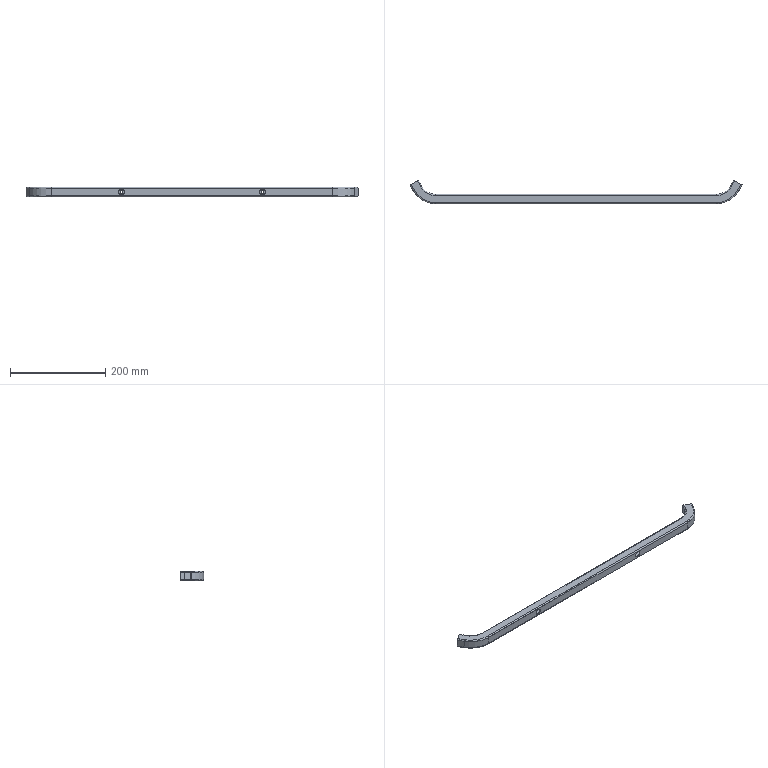Part | STEP file | 7101205 | 1 solid | 70 faces | box 697.147 x 49.49 x 20 mm | volume 75230 mm3 | cylinder 36 | plane 18 | torus 16 | commonest cylinder face diameters 2 x12 5 x12 6 x2 12 x2 66 x2 69 x2